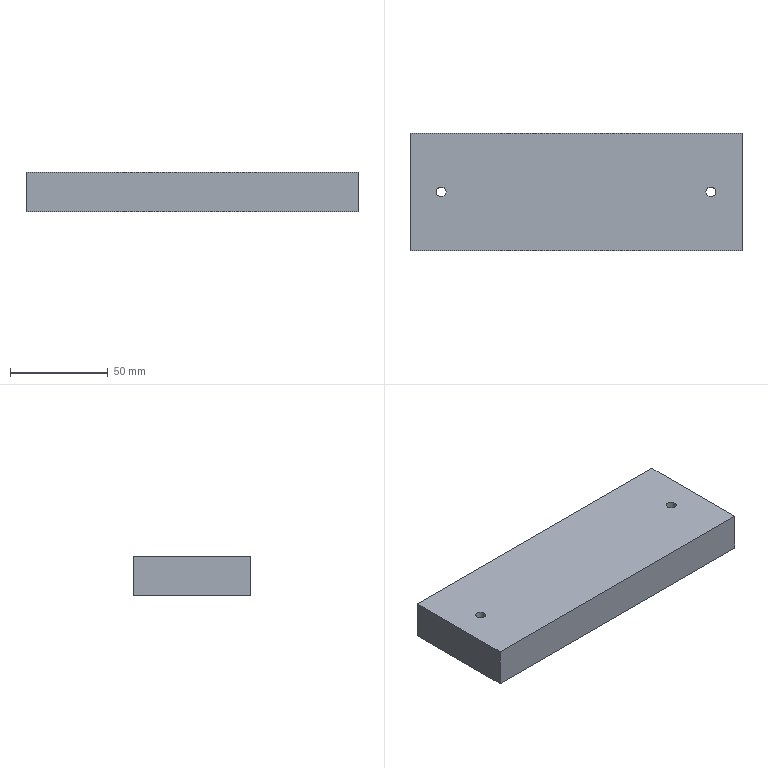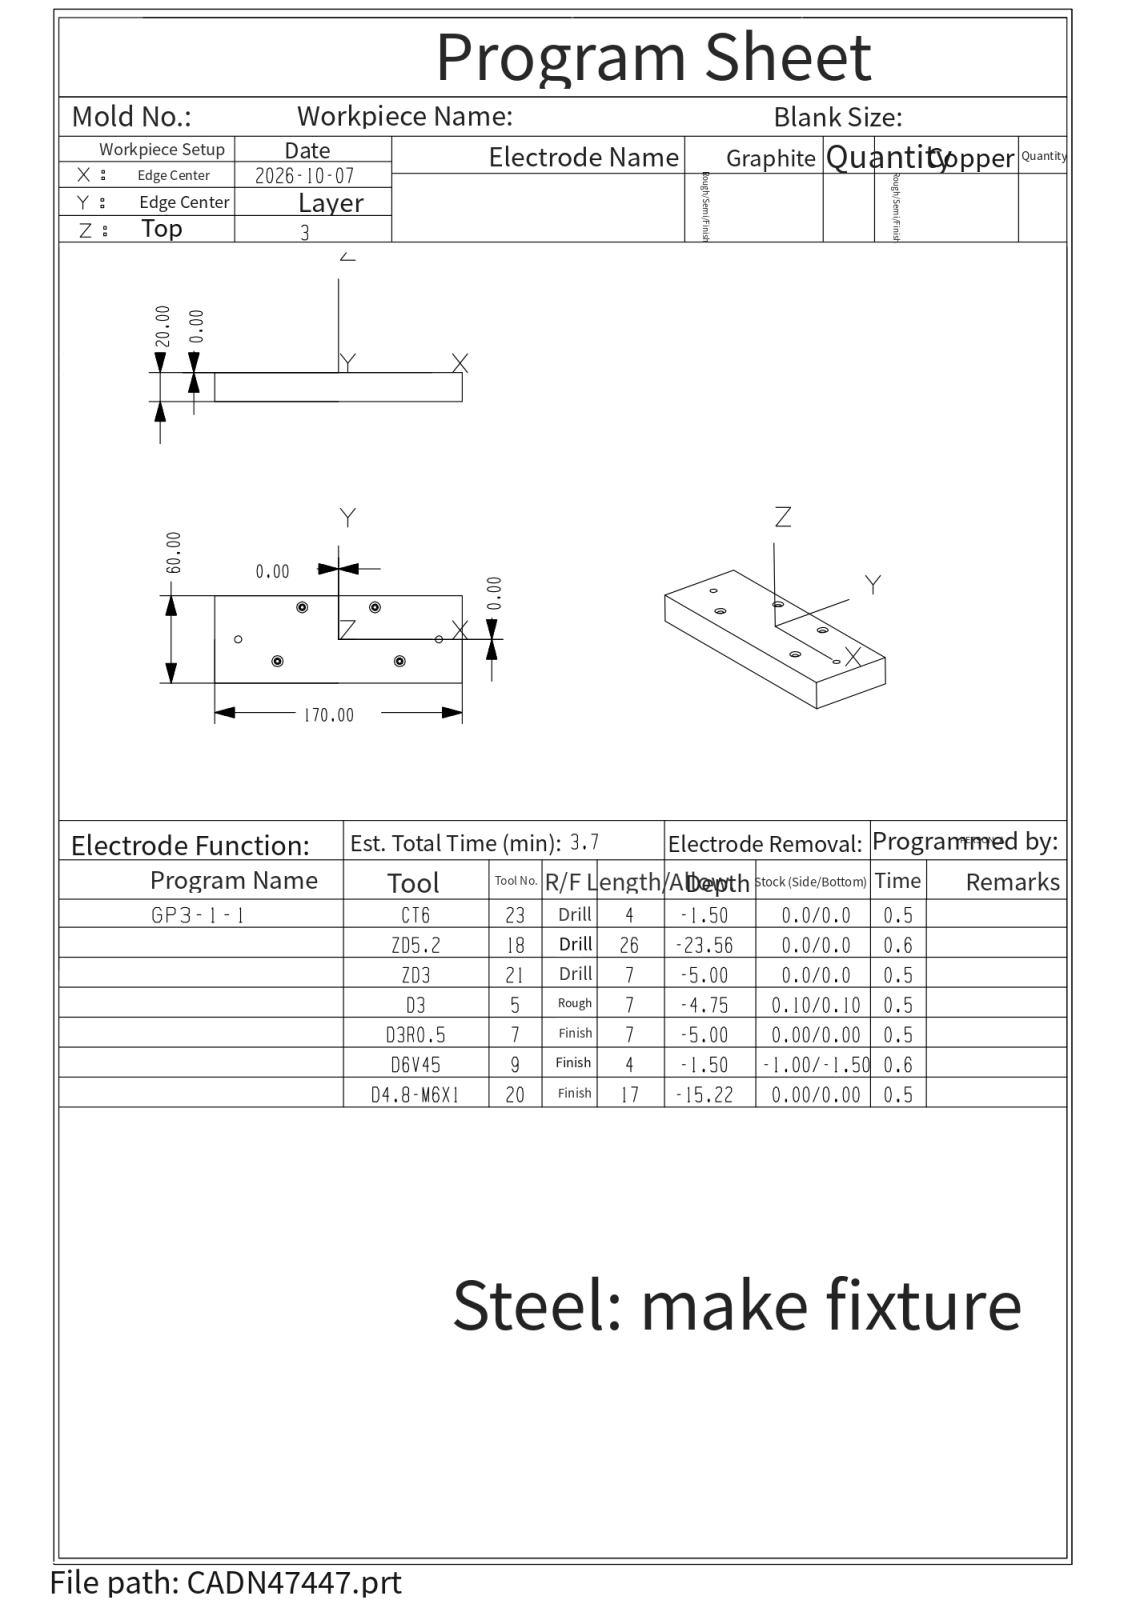NC program | NX | posted by the shop | part box 170 x 60 x 20 mm
Lines 60 to 1040 of 14163:
T05 M06
T07
( name=D3    T=5 )
( XY = 0.10 )
( Z = 0.10 )
G00 G90 G54 X43.611 Y-14.897 S5000 M03
G43 Z10. H05 M08
Z.2
G17 G01 X43.421 Y-14.198 Z.175 F1600.
X43.017 Y-13.724 Z.153
X42.217 Y-13.383 Z.123
X41.354 Y-13.502 Z.092
X40.676 Y-14.048 Z.062
X40.416 Y-14.613 Z.04
X40.389 Y-15.254 Z.018
X40.612 Y-15.855 Z-.005
X41.048 Y-16.325 Z-.027
X41.614 Y-16.585 Z-.049
X41.689 Y-16.601 Z-.052
X42.001 Z-.062
G03 I0.0 J1.601 F2000.
G01 X42.235 Y-16.576 Z-.067
X42.384 Y-16.541 Z-.069
X42.597 Y-16.463 Z-.073
X42.738 Y-16.391 Z-.076
X42.924 Y-16.266 Z-.08
X43.043 Y-16.162 Z-.083
X43.192 Y-15.997 Z-.087
X43.282 Y-15.869 Z-.09
X43.386 Y-15.675 Z-.094
X43.442 Y-15.53 Z-.097
X43.496 Y-15.318 Z-.101
X43.515 Y-15.165 Z-.103
X43.516 Y-14.948 Z-.107
X43.498 Y-14.796 Z-.11
X43.447 Y-14.588 Z-.114
X43.394 Y-14.445 Z-.117
X43.295 Y-14.256 Z-.121
X43.209 Y-14.132 Z-.124
X43.069 Y-13.974 Z-.128
X42.957 Y-13.875 Z-.131
X42.81 Y-13.772 Z-.134
X42.652 Y-13.687 Z-.137
G03 X42.001 Y-16.465 I-.651 J-1.313
G01 X42.256 Y-16.436 Z-.142
X42.406 Y-16.396 Z-.145
X42.629 Y-16.304 Z-.149
X42.772 Y-16.219 Z-.152
X42.958 Y-16.07 Z-.156
X43.073 Y-15.948 Z-.159
X43.208 Y-15.756 Z-.163
X43.284 Y-15.608 Z-.166
X43.361 Y-15.387 Z-.17
X43.392 Y-15.224 Z-.173
X43.404 Y-14.993 Z-.178
X43.389 Y-14.829 Z-.181
X43.336 Y-14.606 Z-.185
X43.277 Y-14.454 Z-.188
X43.165 Y-14.255 Z-.192
X43.067 Y-14.126 Z-.195
X42.905 Y-13.968 Z-.199
X42.776 Y-13.873 Z-.202
X42.577 Y-13.766 Z-.207
X42.428 Y-13.711 Z-.21
X42.21 Y-13.664 Z-.214
X42.052 Y-13.653 Z-.217
X41.863 Y-13.664 Z-.22
X41.677 Y-13.701 Z-.224
G03 X42.001 Y-16.339 I.324 J-1.299
G01 X42.251 Y-16.309 Z-.228
X42.392 Y-16.271 Z-.231
X42.607 Y-16.177 Z-.235
X42.743 Y-16.092 Z-.238
X42.918 Y-15.942 Z-.242
X43.025 Y-15.82 Z-.245
X43.147 Y-15.627 Z-.249
X43.212 Y-15.479 Z-.252
X43.272 Y-15.26 Z-.256
X43.291 Y-15.101 Z-.259
X43.284 Y-14.876 Z-.263
X43.255 Y-14.719 Z-.266
X43.183 Y-14.507 Z-.27
X43.11 Y-14.366 Z-.273
X42.979 Y-14.186 Z-.277
X42.869 Y-14.074 Z-.28
X42.692 Y-13.942 Z-.284
X42.554 Y-13.867 Z-.287
X42.348 Y-13.793 Z-.291
X42.195 Y-13.762 Z-.294
X41.978 Y-13.752 Z-.298
X41.824 Y-13.768 Z-.301
X41.614 Y-13.822 Z-.305
X41.473 Y-13.881 Z-.308
X41.289 Y-13.994 Z-.312
X41.172 Y-14.092 Z-.315
X41.05 Y-14.227 Z-.318
X40.948 Y-14.38 Z-.322
G03 X42.001 Y-16.222 I1.052 J-.62
G01 X42.255 Y-16.189 Z-.327
X42.395 Y-16.147 Z-.33
X42.608 Y-16.043 Z-.335
X42.74 Y-15.95 Z-.338
X42.906 Y-15.786 Z-.343
X43.001 Y-15.653 Z-.347
X43.104 Y-15.447 Z-.351
X43.151 Y-15.291 Z-.355
X43.181 Y-15.064 Z-.36
X43.175 Y-14.902 Z-.363
X43.129 Y-14.68 Z-.368
X43.072 Y-14.53 Z-.371
X42.958 Y-14.335 Z-.376
X42.855 Y-14.213 Z-.38
X42.685 Y-14.067 Z-.385
X42.549 Y-13.985 Z-.388
X42.343 Y-13.903 Z-.393
X42.188 Y-13.87 Z-.396
X41.968 Y-13.86 Z-.401
X41.813 Y-13.878 Z-.405
X41.602 Y-13.939 Z-.41
X41.462 Y-14.007 Z-.413
X41.284 Y-14.132 Z-.418
X41.174 Y-14.241 Z-.421
X41.064 Y-14.389 Z-.425
X40.979 Y-14.553 Z-.43
G03 X42.001 Y-16.115 I1.021 J-.447
G01 X42.253 Y-16.08 Z-.436
X42.389 Y-16.036 Z-.439
X42.597 Y-15.926 Z-.445
X42.723 Y-15.827 Z-.449
X42.875 Y-15.655 Z-.455
X42.96 Y-15.516 Z-.459
X43.041 Y-15.304 Z-.465
X43.072 Y-15.146 Z-.469
X43.074 Y-14.92 Z-.474
X43.047 Y-14.762 Z-.478
X42.97 Y-14.551 Z-.484
X42.89 Y-14.414 Z-.488
X42.745 Y-14.245 Z-.494
X42.622 Y-14.146 Z-.498
X42.429 Y-14.039 Z-.504
X42.281 Y-13.989 Z-.508
X42.064 Y-13.958 Z-.513
X41.908 Y-13.963 Z-.517
X41.696 Y-14.009 Z-.523
X41.553 Y-14.068 Z-.527
X41.372 Y-14.185 Z-.533
X41.26 Y-14.29 Z-.537
X41.148 Y-14.435 Z-.542
X41.064 Y-14.598 Z-.547
G03 X42.001 Y-16.019 I.936 J-.402
G01 X42.254 Y-15.981 Z-.554
X42.388 Y-15.933 Z-.558
X42.59 Y-15.815 Z-.565
X42.71 Y-15.708 Z-.57
X42.849 Y-15.525 Z-.576
X42.92 Y-15.38 Z-.581
X42.977 Y-15.16 Z-.588
X42.987 Y-14.999 Z-.592
X42.957 Y-14.776 Z-.599
X42.904 Y-14.624 Z-.604
X42.791 Y-14.431 Z-.61
X42.686 Y-14.312 Z-.615
X42.509 Y-14.178 Z-.622
X42.368 Y-14.109 Z-.627
X42.155 Y-14.053 Z-.633
X41.998 Y-14.044 Z-.638
X41.782 Y-14.074 Z-.645
X41.635 Y-14.124 Z-.649
X41.448 Y-14.234 Z-.656
X41.333 Y-14.336 Z-.661
X41.219 Y-14.481 Z-.667
X41.136 Y-14.645 Z-.672
G03 X42.001 Y-15.935 I.865 J-.355
G01 X42.258 Y-15.893 Z-.681
X42.391 Y-15.84 Z-.685
X42.59 Y-15.709 Z-.693
X42.703 Y-15.593 Z-.699
X42.826 Y-15.395 Z-.706
X42.88 Y-15.239 Z-.712
X42.908 Y-15.011 Z-.72
X42.892 Y-14.848 Z-.725
X42.821 Y-14.631 Z-.733
X42.739 Y-14.49 Z-.739
X42.584 Y-14.325 Z-.746
X42.452 Y-14.233 Z-.752
X42.244 Y-14.148 Z-.759
X42.086 Y-14.121 Z-.765
X41.863 Y-14.132 Z-.773
X41.71 Y-14.174 Z-.778
X41.514 Y-14.277 Z-.786
X41.393 Y-14.378 Z-.792
X41.277 Y-14.525 Z-.798
X41.194 Y-14.694 Z-.805
G03 X42.001 Y-15.863 I.807 J-.306
G01 X42.268 Y-15.816 Z-.815
X42.402 Y-15.756 Z-.82
X42.598 Y-15.606 Z-.829
X42.703 Y-15.476 Z-.836
X42.805 Y-15.257 Z-.845
X42.837 Y-15.09 Z-.851
X42.825 Y-14.852 Z-.86
X42.776 Y-14.69 Z-.866
X42.655 Y-14.487 Z-.875
X42.536 Y-14.368 Z-.882
X42.336 Y-14.247 Z-.891
X42.176 Y-14.197 Z-.897
X41.944 Y-14.184 Z-.906
X41.781 Y-14.215 Z-.913
X41.571 Y-14.311 Z-.922
X41.442 Y-14.414 Z-.928
X41.32 Y-14.567 Z-.936
X41.238 Y-14.746 Z-.943
G03 X42.001 Y-15.804 I.763 J-.254
G01 X42.254 Y-15.759 Z-.954
X42.379 Y-15.703 Z-.959
X42.564 Y-15.561 Z-.969
X42.662 Y-15.436 Z-.975
X42.756 Y-15.229 Z-.984
X42.785 Y-15.07 Z-.991
X42.769 Y-14.845 Z-1.
X42.719 Y-14.692 Z-1.007
X42.6 Y-14.503 Z-1.016
X42.484 Y-14.392 Z-1.023
X42.291 Y-14.283 Z-1.032
X42.138 Y-14.24 Z-1.039
X41.917 Y-14.236 Z-1.048
X41.763 Y-14.271 Z-1.055
X41.567 Y-14.371 Z-1.064
X41.449 Y-14.474 Z-1.071
X41.339 Y-14.625 Z-1.079
X41.27 Y-14.8 Z-1.087
G03 X42.001 Y-15.758 I.731 J-.2
G01 X42.244 Y-15.715 Z-1.097
X42.363 Y-15.661 Z-1.103
X42.54 Y-15.523 Z-1.113
X42.633 Y-15.403 Z-1.119
X42.721 Y-15.202 Z-1.129
X42.745 Y-15.049 Z-1.136
X42.726 Y-14.833 Z-1.145
X42.674 Y-14.687 Z-1.152
X42.553 Y-14.508 Z-1.161
X42.438 Y-14.405 Z-1.168
X42.247 Y-14.306 Z-1.178
X42.098 Y-14.271 Z-1.185
X41.884 Y-14.276 Z-1.194
X41.737 Y-14.317 Z-1.201
X41.552 Y-14.424 Z-1.21
X41.443 Y-14.53 Z-1.217
X41.346 Y-14.684 Z-1.225
X41.289 Y-14.857 Z-1.233
G03 X42.001 Y-15.726 I.712 J-.143
G01 X42.267 Y-15.674 Z-1.246
X42.392 Y-15.608 Z-1.252
X42.519 Y-15.503 Z-1.259
X42.572 Y-15.441 Z-1.263
X42.603 Y-15.396 Z-1.266
X42.656 Y-15.299 Z-1.271
X42.707 Y-15.138 Z-1.278
X42.717 Y-15.057 Z-1.282
X42.719 Y-15.004 Z-1.284
X42.711 Y-14.897 Z-1.289
X42.632 Y-14.661 Z-1.3
X42.541 Y-14.531 Z-1.308
X42.421 Y-14.423 Z-1.315
X42.355 Y-14.38 Z-1.319
X42.305 Y-14.355 Z-1.321
X42.2 Y-14.316 Z-1.326
X41.955 Y-14.29 Z-1.337
X41.799 Y-14.319 Z-1.345
X41.587 Y-14.425 Z-1.356
X41.465 Y-14.538 Z-1.363
X41.358 Y-14.708 Z-1.373
X41.303 Y-14.902 Z-1.382
G03 X42.001 Y-15.705 I.698 J-.098
G01 X42.26 Y-15.654 Z-1.394
X42.381 Y-15.591 Z-1.401
X42.555 Y-15.429 Z-1.412
X42.637 Y-15.29 Z-1.419
X42.696 Y-15.065 Z-1.43
X42.691 Y-14.9 Z-1.438
X42.618 Y-14.68 Z-1.448
X42.525 Y-14.544 Z-1.456
X42.346 Y-14.399 Z-1.467
X42.194 Y-14.336 Z-1.475
X41.967 Y-14.311 Z-1.486
X41.805 Y-14.339 Z-1.493
X41.601 Y-14.441 Z-1.504
X41.481 Y-14.552 Z-1.512
X41.377 Y-14.717 Z-1.521
X41.324 Y-14.905 Z-1.531
G03 X42.001 Y-15.684 I.677 J-.095
G01 X42.252 Y-15.634 Z-1.543
X42.369 Y-15.573 Z-1.549
X42.538 Y-15.416 Z-1.56
X42.618 Y-15.282 Z-1.568
X42.675 Y-15.064 Z-1.578
X42.67 Y-14.904 Z-1.586
X42.601 Y-14.691 Z-1.597
X42.51 Y-14.559 Z-1.605
X42.337 Y-14.418 Z-1.616
X42.19 Y-14.356 Z-1.623
X41.97 Y-14.331 Z-1.634
X41.813 Y-14.359 Z-1.642
X41.615 Y-14.456 Z-1.653
X41.498 Y-14.564 Z-1.66
X41.397 Y-14.723 Z-1.67
X41.345 Y-14.905 Z-1.679
G03 X42.001 Y-15.663 I.656 J-.095
G01 X42.244 Y-15.615 Z-1.691
X42.357 Y-15.556 Z-1.698
X42.521 Y-15.404 Z-1.709
X42.599 Y-15.274 Z-1.716
X42.654 Y-15.063 Z-1.727
X42.65 Y-14.908 Z-1.735
X42.583 Y-14.702 Z-1.746
X42.495 Y-14.574 Z-1.753
X42.328 Y-14.437 Z-1.764
X42.186 Y-14.377 Z-1.772
X41.973 Y-14.352 Z-1.783
X41.821 Y-14.378 Z-1.79
X41.629 Y-14.472 Z-1.801
X41.516 Y-14.575 Z-1.809
X41.417 Y-14.729 Z-1.818
X41.366 Y-14.905 Z-1.828
G03 X42.001 Y-15.642 I.635 J-.095
G01 X42.185 Y-15.614 Z-1.837
X42.267 Y-15.582 Z-1.841
X42.309 Y-15.561 Z-1.844
X42.388 Y-15.508 Z-1.849
X42.509 Y-15.385 Z-1.857
X42.555 Y-15.316 Z-1.862
X42.578 Y-15.269 Z-1.864
X42.614 Y-15.169 Z-1.87
X42.636 Y-15. Z-1.879
X42.63 Y-14.918 Z-1.883
X42.62 Y-14.866 Z-1.886
X42.588 Y-14.763 Z-1.891
X42.503 Y-14.617 Z-1.9
X42.449 Y-14.556 Z-1.904
X42.41 Y-14.52 Z-1.907
X42.323 Y-14.458 Z-1.912
X42.167 Y-14.393 Z-1.921
X42.088 Y-14.378 Z-1.925
X42.035 Y-14.373 Z-1.928
X41.929 Y-14.377 Z-1.934
X41.767 Y-14.419 Z-1.942
X41.694 Y-14.455 Z-1.946
X41.65 Y-14.483 Z-1.949
X41.568 Y-14.55 Z-1.955
X41.501 Y-14.628 Z-1.96
X41.448 Y-14.713 Z-1.966
X41.41 Y-14.805 Z-1.971
X41.387 Y-14.905 Z-1.976
G03 X42.001 Y-15.621 I.614 J-.095
G01 X42.178 Y-15.594 Z-1.985
X42.258 Y-15.563 Z-1.99
X42.299 Y-15.543 Z-1.992
X42.375 Y-15.492 Z-1.997
X42.492 Y-15.373 Z-2.006
X42.536 Y-15.306 Z-2.01
X42.559 Y-15.261 Z-2.013
X42.594 Y-15.164 Z-2.019
X42.615 Y-15.001 Z-2.027
X42.609 Y-14.922 Z-2.031
X42.6 Y-14.871 Z-2.034
X42.569 Y-14.772 Z-2.04
X42.488 Y-14.631 Z-2.048
X42.436 Y-14.571 Z-2.053
X42.398 Y-14.537 Z-2.055
X42.314 Y-14.477 Z-2.061
X42.164 Y-14.414 Z-2.07
X42.087 Y-14.399 Z-2.074
X42.036 Y-14.394 Z-2.077
X41.933 Y-14.397 Z-2.082
X41.777 Y-14.438 Z-2.091
X41.707 Y-14.472 Z-2.095
X41.664 Y-14.499 Z-2.098
X41.584 Y-14.563 Z-2.103
X41.519 Y-14.638 Z-2.109
X41.468 Y-14.72 Z-2.114
X41.431 Y-14.809 Z-2.119
X41.408 Y-14.905 Z-2.125
G03 X42.001 Y-15.6 I.593 J-.095
G01 X42.172 Y-15.574 Z-2.134
X42.249 Y-15.545 Z-2.138
X42.288 Y-15.524 Z-2.141
X42.362 Y-15.476 Z-2.146
X42.475 Y-15.361 Z-2.154
X42.518 Y-15.296 Z-2.159
X42.54 Y-15.252 Z-2.162
X42.574 Y-15.159 Z-2.167
X42.594 Y-15.002 Z-2.176
X42.589 Y-14.926 Z-2.18
X42.58 Y-14.877 Z-2.183
X42.55 Y-14.781 Z-2.188
X42.472 Y-14.644 Z-2.197
X42.422 Y-14.587 Z-2.201
X42.386 Y-14.554 Z-2.204
X42.305 Y-14.496 Z-2.21
X42.16 Y-14.435 Z-2.218
X42.086 Y-14.42 Z-2.222
X42.037 Y-14.415 Z-2.225
X41.938 Y-14.418 Z-2.231
X41.787 Y-14.456 Z-2.239
X41.719 Y-14.489 Z-2.244
X41.677 Y-14.515 Z-2.246
X41.601 Y-14.577 Z-2.252
X41.538 Y-14.648 Z-2.257
X41.488 Y-14.727 Z-2.263
X41.452 Y-14.812 Z-2.268
X41.429 Y-14.905 Z-2.273
G03 X42.001 Y-15.58 I.572 J-.095
G01 X42.166 Y-15.554 Z-2.282
X42.278 Y-15.506 Z-2.289
X42.349 Y-15.459 Z-2.294
X42.458 Y-15.349 Z-2.303
X42.499 Y-15.287 Z-2.307
X42.521 Y-15.244 Z-2.31
X42.553 Y-15.155 Z-2.316
X42.573 Y-15.003 Z-2.324
X42.568 Y-14.93 Z-2.328
X42.56 Y-14.882 Z-2.331
X42.532 Y-14.79 Z-2.337
X42.456 Y-14.658 Z-2.345
X42.408 Y-14.603 Z-2.35
X42.373 Y-14.571 Z-2.352
X42.295 Y-14.515 Z-2.358
X42.156 Y-14.455 Z-2.367
X42.085 Y-14.441 Z-2.371
X42.038 Y-14.436 Z-2.374
X41.943 Y-14.438 Z-2.379
X41.797 Y-14.475 Z-2.388
X41.731 Y-14.506 Z-2.392
X41.691 Y-14.53 Z-2.395
X41.617 Y-14.59 Z-2.401
X41.508 Y-14.734 Z-2.411
X41.45 Y-14.906 Z-2.422
G03 X42.001 Y-15.559 I.551 J-.094
G01 X42.186 Y-15.525 Z-2.432
X42.266 Y-15.489 Z-2.438
X42.307 Y-15.464 Z-2.441
X42.382 Y-15.404 Z-2.447
X42.487 Y-15.265 Z-2.456
X42.52 Y-15.189 Z-2.461
X42.536 Y-15.139 Z-2.465
X42.552 Y-15.032 Z-2.471
X42.533 Y-14.862 Z-2.481
X42.507 Y-14.785 Z-2.486
X42.483 Y-14.737 Z-2.489
X42.421 Y-14.648 Z-2.496
X42.292 Y-14.537 Z-2.506
X42.22 Y-14.5 Z-2.511
X42.17 Y-14.481 Z-2.514
X42.065 Y-14.459 Z-2.521
X41.895 Y-14.467 Z-2.531
X41.818 Y-14.489 Z-2.536
X41.77 Y-14.51 Z-2.539
X41.678 Y-14.565 Z-2.546
X41.602 Y-14.635 Z-2.552
X41.542 Y-14.716 Z-2.558
X41.498 Y-14.806 Z-2.564
X41.471 Y-14.906 Z-2.57
G03 X42.001 Y-15.538 I.529 J-.094
G01 X42.179 Y-15.506 Z-2.581
X42.256 Y-15.471 Z-2.586
X42.295 Y-15.447 Z-2.589
X42.367 Y-15.389 Z-2.595
X42.468 Y-15.256 Z-2.605
X42.5 Y-15.183 Z-2.61
X42.515 Y-15.134 Z-2.613
X42.531 Y-15.032 Z-2.62
X42.514 Y-14.868 Z-2.63
X42.488 Y-14.794 Z-2.635
X42.465 Y-14.748 Z-2.638
X42.406 Y-14.663 Z-2.645
X42.282 Y-14.556 Z-2.654
X42.214 Y-14.52 Z-2.659
X42.166 Y-14.502 Z-2.663
X42.065 Y-14.48 Z-2.669
X41.902 Y-14.487 Z-2.679
X41.828 Y-14.508 Z-2.684
X41.781 Y-14.527 Z-2.687
X41.693 Y-14.58 Z-2.694
X41.62 Y-14.647 Z-2.7
X41.562 Y-14.724 Z-2.706
X41.519 Y-14.81 Z-2.713
X41.493 Y-14.906 Z-2.719
G03 X42.001 Y-15.517 I.508 J-.094
G01 X42.172 Y-15.486 Z-2.729
X42.245 Y-15.453 Z-2.735
X42.283 Y-15.43 Z-2.738
X42.352 Y-15.374 Z-2.744
X42.45 Y-15.246 Z-2.754
X42.481 Y-15.177 Z-2.759
X42.495 Y-15.13 Z-2.762
X42.51 Y-15.032 Z-2.768
X42.494 Y-14.875 Z-2.778
X42.469 Y-14.804 Z-2.783
X42.448 Y-14.76 Z-2.786
X42.391 Y-14.678 Z-2.793
X42.273 Y-14.574 Z-2.803
X42.207 Y-14.54 Z-2.808
X42.161 Y-14.522 Z-2.811
X42.064 Y-14.501 Z-2.818
X41.909 Y-14.507 Z-2.828
X41.838 Y-14.526 Z-2.833
X41.792 Y-14.545 Z-2.836
X41.708 Y-14.595 Z-2.843
X41.637 Y-14.659 Z-2.849
X41.581 Y-14.732 Z-2.855
X41.54 Y-14.814 Z-2.861
X41.514 Y-14.906 Z-2.867
G03 X42.001 Y-15.496 I.487 J-.094
G01 X42.164 Y-15.467 Z-2.878
X42.235 Y-15.435 Z-2.883
X42.271 Y-15.413 Z-2.886
X42.337 Y-15.36 Z-2.892
X42.431 Y-15.237 Z-2.902
X42.461 Y-15.171 Z-2.907
X42.474 Y-15.126 Z-2.91
X42.489 Y-15.032 Z-2.917
X42.474 Y-14.882 Z-2.927
X42.451 Y-14.814 Z-2.932
X42.43 Y-14.771 Z-2.935
X42.376 Y-14.692 Z-2.942
X42.264 Y-14.593 Z-2.952
X42.201 Y-14.56 Z-2.956
X42.157 Y-14.543 Z-2.96
X42.064 Y-14.522 Z-2.966
X41.915 Y-14.527 Z-2.976
X41.847 Y-14.545 Z-2.981
X41.804 Y-14.563 Z-2.985
X41.723 Y-14.61 Z-2.991
X41.655 Y-14.671 Z-2.997
X41.601 Y-14.74 Z-3.004
X41.561 Y-14.819 Z-3.01
X41.535 Y-14.906 Z-3.016
G03 X42.001 Y-15.475 I.466 J-.094
G01 X42.157 Y-15.447 Z-3.027
X42.225 Y-15.417 Z-3.032
X42.259 Y-15.396 Z-3.035
X42.323 Y-15.345 Z-3.041
X42.412 Y-15.228 Z-3.051
X42.441 Y-15.165 Z-3.056
X42.454 Y-15.122 Z-3.059
X42.468 Y-15.032 Z-3.065
X42.454 Y-14.888 Z-3.075
X42.432 Y-14.823 Z-3.08
X42.413 Y-14.783 Z-3.084
X42.362 Y-14.707 Z-3.09
X42.254 Y-14.612 Z-3.1
X42.194 Y-14.58 Z-3.105
X42.153 Y-14.563 Z-3.108
X42.064 Y-14.543 Z-3.115
X41.922 Y-14.547 Z-3.125
X41.857 Y-14.564 Z-3.13
X41.815 Y-14.58 Z-3.133
X41.738 Y-14.626 Z-3.14
X41.672 Y-14.683 Z-3.146
X41.62 Y-14.749 Z-3.152
X41.581 Y-14.823 Z-3.158
X41.556 Y-14.907 Z-3.164
G03 X42.001 Y-15.454 I.445 J-.093
G01 X42.179 Y-15.416 Z-3.177
X42.252 Y-15.375 Z-3.183
X42.289 Y-15.347 Z-3.187
X42.353 Y-15.28 Z-3.194
X42.43 Y-15.13 Z-3.206
X42.445 Y-15.054 Z-3.212
X42.448 Y-15.003 Z-3.216
X42.435 Y-14.899 Z-3.224
X42.367 Y-14.749 Z-3.236
X42.318 Y-14.69 Z-3.242
X42.28 Y-14.656 Z-3.246
X42.191 Y-14.601 Z-3.254
X42.032 Y-14.561 Z-3.265
X41.956 Y-14.563 Z-3.271
X41.906 Y-14.572 Z-3.275
X41.808 Y-14.607 Z-3.283
X41.725 Y-14.662 Z-3.291
X41.659 Y-14.73 Z-3.298
X41.609 Y-14.812 Z-3.306
X41.578 Y-14.907 Z-3.313
G03 X42.001 Y-15.433 I.423 J-.093
G01 X42.171 Y-15.397 Z-3.326
X42.24 Y-15.358 Z-3.332
X42.275 Y-15.332 Z-3.336
X42.336 Y-15.268 Z-3.343
X42.41 Y-15.125 Z-3.355
X42.424 Y-15.053 Z-3.36
X42.427 Y-15.004 Z-3.364
X42.415 Y-14.906 Z-3.372
X42.351 Y-14.762 Z-3.384
X42.305 Y-14.706 Z-3.39
X42.268 Y-14.674 Z-3.394
X42.184 Y-14.621 Z-3.402
X42.033 Y-14.582 Z-3.414
X41.962 Y-14.583 Z-3.42
X41.914 Y-14.591 Z-3.424
X41.821 Y-14.624 Z-3.432
X41.741 Y-14.676 Z-3.439
X41.678 Y-14.74 Z-3.447
X41.63 Y-14.817 Z-3.454
X41.599 Y-14.907 Z-3.462
G03 X42.001 Y-15.413 I.402 J-.093
G01 X42.162 Y-15.378 Z-3.474
X42.228 Y-15.341 Z-3.48
X42.261 Y-15.316 Z-3.484
X42.319 Y-15.256 Z-3.491
X42.389 Y-15.12 Z-3.503
X42.403 Y-15.052 Z-3.509
X42.406 Y-15.005 Z-3.513
X42.395 Y-14.912 Z-3.521
X42.335 Y-14.776 Z-3.533
X42.291 Y-14.723 Z-3.539
X42.257 Y-14.691 Z-3.543
X42.177 Y-14.641 Z-3.551
X42.035 Y-14.603 Z-3.562
X41.967 Y-14.604 Z-3.568
X41.921 Y-14.611 Z-3.572
X41.833 Y-14.641 Z-3.58
X41.757 Y-14.689 Z-3.588
X41.697 Y-14.75 Z-3.595
X41.651 Y-14.822 Z-3.603
X41.62 Y-14.907 Z-3.61
G03 X42.001 Y-15.392 I.381 J-.093
G01 X42.153 Y-15.359 Z-3.623
X42.215 Y-15.324 Z-3.629
X42.247 Y-15.301 Z-3.633
X42.302 Y-15.243 Z-3.64
X42.369 Y-15.116 Z-3.652
X42.382 Y-15.051 Z-3.658
X42.385 Y-15.007 Z-3.662
X42.375 Y-14.919 Z-3.669
X42.319 Y-14.789 Z-3.681
X42.278 Y-14.739 Z-3.687
X42.246 Y-14.709 Z-3.691
X42.171 Y-14.661 Z-3.699
X42.036 Y-14.624 Z-3.711
X41.972 Z-3.717
X41.929 Y-14.631 Z-3.721
X41.845 Y-14.659 Z-3.729
X41.773 Y-14.703 Z-3.736
X41.716 Y-14.76 Z-3.744
X41.671 Y-14.828 Z-3.751
X41.642 Y-14.908 Z-3.759
G03 X42.001 Y-15.371 I.359 J-.092
G01 X42.18 Y-15.322 Z-3.774
X42.245 Y-15.275 Z-3.782
X42.277 Y-15.241 Z-3.786
X42.329 Y-15.162 Z-3.796
X42.364 Y-14.996 Z-3.81
X42.355 Y-14.922 Z-3.818
X42.339 Y-14.872 Z-3.823
X42.287 Y-14.781 Z-3.833
X42.157 Y-14.678 Z-3.847
X42.088 Y-14.654 Z-3.854
X42.038 Y-14.645 Z-3.86
X41.932 Y-14.652 Z-3.87
X41.838 Y-14.686 Z-3.879
X41.762 Y-14.741 Z-3.889
X41.703 Y-14.814 Z-3.898
X41.663 Y-14.908 Z-3.907
G03 X42.001 Y-15.35 I.338 J-.092
G01 X42.169 Y-15.304 Z-3.923
X42.23 Y-15.26 Z-3.93
X42.261 Y-15.229 Z-3.935
X42.309 Y-15.154 Z-3.944
X42.343 Y-14.998 Z-3.959
X42.335 Y-14.928 Z-3.966
X42.321 Y-14.882 Z-3.971
X42.272 Y-14.796 Z-3.981
X42.151 Y-14.698 Z-3.996
X42.087 Y-14.675 Z-4.003
X42.039 Y-14.666 Z-4.008
X41.94 Y-14.671 Z-4.019
X41.851 Y-14.703 Z-4.028
X41.779 Y-14.753 Z-4.037
X41.723 Y-14.821 Z-4.046
X41.685 Y-14.909 Z-4.056
G03 X42.001 Y-15.329 I.316 J-.091
G01 X42.158 Y-15.286 Z-4.071
X42.215 Y-15.245 Z-4.079
X42.244 Y-15.216 Z-4.084
X42.29 Y-15.146 Z-4.093
X42.323 Y-15. Z-4.107
X42.315 Y-14.935 Z-4.115
X42.302 Y-14.892 Z-4.12
X42.257 Y-14.811 Z-4.13
X42.145 Y-14.718 Z-4.144
X42.085 Y-14.696 Z-4.152
X42.04 Y-14.688 Z-4.157
X41.948 Y-14.691 Z-4.167
X41.865 Y-14.719 Z-4.176
X41.797 Y-14.765 Z-4.186
X41.743 Y-14.828 Z-4.195
X41.706 Y-14.909 Z-4.204
G03 X42.001 Y-15.308 I.294 J-.091
G01 X42.147 Y-15.269 Z-4.22
X42.201 Y-15.23 Z-4.227
X42.228 Y-15.203 Z-4.232
X42.271 Y-15.138 Z-4.241
X42.302 Y-15.002 Z-4.256
X42.295 Y-14.942 Z-4.263
X42.283 Y-14.901 Z-4.268
X42.242 Y-14.826 Z-4.278
X42.139 Y-14.738 Z-4.293
X42.083 Y-14.717 Z-4.3
X42.042 Y-14.709 Z-4.305
X41.956 Y-14.711 Z-4.316
X41.878 Y-14.736 Z-4.325
X41.815 Y-14.778 Z-4.334
X41.764 Y-14.835 Z-4.343
X41.728 Y-14.91 Z-4.353
G03 X42.001 Y-15.287 I.273 J-.09
G01 X42.18 Y-15.221 Z-4.372
X42.229 Y-15.167 Z-4.382
X42.253 Y-15.126 Z-4.389
X42.276 Y-15.055 Z-4.399
X42.279 Y-15.032 Z-4.402
X42.236 Y-14.853 Z-4.422
X42.19 Y-14.799 Z-4.431
X42.153 Y-14.77 Z-4.438
X42.085 Y-14.74 Z-4.448
X42.063 Y-14.734 Z-4.452
X41.959 Y-14.732 Z-4.464
X41.873 Y-14.762 Z-4.477
X41.803 Y-14.82 Z-4.489
X41.75 Y-14.911 Z-4.501
G03 X42.001 Y-15.266 I.251 J-.089
G01 X42.164 Y-15.207 Z-4.518
X42.21 Y-15.159 Z-4.526
X42.233 Y-15.122 Z-4.532
X42.259 Y-15.037 Z-4.543
X42.231 Y-14.882 Z-4.558
X42.195 Y-14.831 Z-4.566
X42.16 Y-14.799 Z-4.572
X42.096 Y-14.764 Z-4.581
X42.072 Y-14.757 Z-4.584
X41.979 Y-14.75 Z-4.595
X41.901 Y-14.773 Z-4.605
X41.833 Y-14.821 Z-4.616
X41.78 Y-14.9 Z-4.626
G03 X42.001 Y-15.242 I.221 J-.1
G01 X41.794 Y-15.06 Z-4.688
X41.958 Y-14.831 Z-4.751
G03 I.043 J-.169
G01 Z-3.751
G00 Z10.
X23.395 Y21.889
Z.2
G01 X23.389 Y21.746 Z.195 F1600.
X23.612 Y21.145 Z.173
X24.048 Y20.675 Z.15
X24.614 Y20.415 Z.128
X25.337 Y20.404 Z.103
X25.911 Y20.646 Z.081
X26.447 Y21.245 Z.053
X26.632 Y22.027 Z.025
X26.421 Y22.802 Z-.003
X26.017 Y23.276 Z-.024
X25.312 Y23.601 Z-.052
X25.001 Z-.062
G03 I0.0 J-1.601 F2000.
G01 X24.766 Y23.576 Z-.067
X24.618 Y23.541 Z-.069
X24.404 Y23.463 Z-.073
X24.263 Y23.391 Z-.076
X24.078 Y23.266 Z-.08
X23.958 Y23.162 Z-.083
X23.81 Y22.997 Z-.087
X23.719 Y22.869 Z-.09
X23.616 Y22.675 Z-.094
X23.559 Y22.53 Z-.097
X23.506 Y22.318 Z-.101
X23.486 Y22.165 Z-.103
X23.485 Y21.948 Z-.107
X23.503 Y21.796 Z-.11
X23.554 Y21.588 Z-.114
X23.608 Y21.445 Z-.117
X23.707 Y21.256 Z-.121
X23.792 Y21.132 Z-.124
X23.933 Y20.974 Z-.128
X24.045 Y20.875 Z-.131
X24.191 Y20.772 Z-.134
X24.35 Y20.687 Z-.137
G03 X25.001 Y23.465 I.651 J1.313
G01 X24.746 Y23.436 Z-.142
X24.596 Y23.396 Z-.145
X24.373 Y23.304 Z-.149
X24.229 Y23.219 Z-.152
X24.044 Y23.07 Z-.156
X23.929 Y22.948 Z-.159
X23.793 Y22.756 Z-.163
X23.717 Y22.608 Z-.166
X23.641 Y22.387 Z-.17
X23.609 Y22.224 Z-.173
X23.598 Y21.993 Z-.178
X23.613 Y21.829 Z-.181
X23.665 Y21.606 Z-.185
X23.725 Y21.454 Z-.188
X23.837 Y21.255 Z-.192
X23.935 Y21.126 Z-.195
X24.097 Y20.968 Z-.199
X24.226 Y20.873 Z-.202
X24.424 Y20.766 Z-.207
X24.574 Y20.711 Z-.21
X24.792 Y20.664 Z-.214
X24.95 Y20.653 Z-.217
X25.139 Y20.664 Z-.22
X25.325 Y20.701 Z-.224
G03 X25.001 Y23.339 I-.324 J1.299
G01 X24.75 Y23.309 Z-.228
X24.61 Y23.271 Z-.231
X24.395 Y23.177 Z-.235
X24.258 Y23.092 Z-.238
X24.083 Y22.942 Z-.242
X23.977 Y22.82 Z-.245
X23.855 Y22.627 Z-.249
X23.789 Y22.479 Z-.252
X23.729 Y22.26 Z-.256
X23.711 Y22.101 Z-.259
X23.718 Y21.876 Z-.263
X23.746 Y21.719 Z-.266
X23.819 Y21.507 Z-.27
X23.892 Y21.366 Z-.273
X24.022 Y21.186 Z-.277
X24.133 Y21.074 Z-.28
X24.31 Y20.942 Z-.284
X24.447 Y20.867 Z-.287
X24.654 Y20.793 Z-.291
X24.806 Y20.762 Z-.294
X25.024 Y20.752 Z-.298
X25.178 Y20.768 Z-.301
X25.388 Y20.822 Z-.305
X25.529 Y20.881 Z-.308
X25.713 Y20.994 Z-.312
X25.829 Y21.092 Z-.315
X25.952 Y21.227 Z-.318
X26.053 Y21.38 Z-.322
G03 X25.001 Y23.222 I-1.052 J.62
G01 X24.747 Y23.189 Z-.327
X24.607 Y23.147 Z-.33
X24.394 Y23.043 Z-.335
X24.261 Y22.95 Z-.338
X24.096 Y22.786 Z-.343
X24. Y22.653 Z-.347
X23.898 Y22.447 Z-.351
X23.851 Y22.291 Z-.355
X23.821 Y22.064 Z-.36
X23.827 Y21.902 Z-.363
X23.872 Y21.68 Z-.368
X23.93 Y21.53 Z-.371
X24.044 Y21.335 Z-.376
X24.147 Y21.213 Z-.38
X24.317 Y21.067 Z-.385
X24.453 Y20.985 Z-.388
X24.659 Y20.903 Z-.393
X24.813 Y20.87 Z-.396
X25.034 Y20.86 Z-.401
X25.189 Y20.878 Z-.405
X25.399 Y20.939 Z-.41
X25.54 Y21.007 Z-.413
X25.717 Y21.132 Z-.418
X25.827 Y21.241 Z-.421
X25.938 Y21.389 Z-.425
X26.022 Y21.553 Z-.43
G03 X25.001 Y23.115 I-1.021 J.447
G01 X24.749 Y23.08 Z-.436
X24.612 Y23.036 Z-.439
X24.405 Y22.926 Z-.445
X24.279 Y22.827 Z-.449
X24.126 Y22.655 Z-.455
X24.042 Y22.516 Z-.459
X23.96 Y22.304 Z-.465
X23.93 Y22.146 Z-.469
X23.928 Y21.92 Z-.474
X23.955 Y21.762 Z-.478
X24.032 Y21.551 Z-.484
X24.112 Y21.414 Z-.488
X24.257 Y21.245 Z-.494
X24.379 Y21.146 Z-.498
X24.572 Y21.039 Z-.504
X24.721 Y20.989 Z-.508
X24.938 Y20.958 Z-.513
X25.093 Y20.963 Z-.517
X25.306 Y21.009 Z-.523
X25.448 Y21.068 Z-.527
X25.63 Y21.185 Z-.533
X25.742 Y21.29 Z-.537
X25.853 Y21.435 Z-.542
X25.937 Y21.598 Z-.547
G03 X25.001 Y23.019 I-.936 J.402
G01 X24.748 Y22.981 Z-.554
X24.614 Y22.933 Z-.558
X24.411 Y22.815 Z-.565
X24.292 Y22.708 Z-.57
X24.153 Y22.525 Z-.576
X24.082 Y22.38 Z-.581
X24.024 Y22.16 Z-.588
X24.015 Y21.999 Z-.592
X24.045 Y21.776 Z-.599
X24.097 Y21.624 Z-.604
X24.21 Y21.431 Z-.61
X24.316 Y21.312 Z-.615
X24.492 Y21.178 Z-.622
X24.634 Y21.109 Z-.627
X24.847 Y21.053 Z-.633
X25.003 Y21.044 Z-.638
X25.22 Y21.074 Z-.645
X25.366 Y21.124 Z-.649
X25.553 Y21.234 Z-.656
X25.669 Y21.336 Z-.661
X25.782 Y21.481 Z-.667
X25.866 Y21.645 Z-.672
G03 X25.001 Y22.935 I-.865 J.355
G01 X24.743 Y22.893 Z-.681
X24.61 Y22.84 Z-.685
X24.411 Y22.709 Z-.693
X24.298 Y22.593 Z-.699
X24.176 Y22.395 Z-.706
X24.121 Y22.239 Z-.712
X24.094 Y22.011 Z-.72
X24.11 Y21.848 Z-.725
X24.18 Y21.631 Z-.733
X24.263 Y21.49 Z-.739
X24.417 Y21.325 Z-.746
X24.55 Y21.233 Z-.752
X24.758 Y21.148 Z-.759
X24.916 Y21.121 Z-.765
X25.139 Y21.132 Z-.773
X25.292 Y21.174 Z-.778
X25.488 Y21.277 Z-.786
X25.608 Y21.378 Z-.792
X25.725 Y21.525 Z-.798
X25.808 Y21.694 Z-.805
G03 X25.001 Y22.863 I-.807 J.306
G01 X24.734 Y22.816 Z-.815
X24.6 Y22.756 Z-.82
X24.403 Y22.606 Z-.829
X24.298 Y22.476 Z-.836
X24.197 Y22.257 Z-.845
X24.164 Y22.09 Z-.851
X24.176 Y21.852 Z-.86
X24.226 Y21.69 Z-.866
X24.347 Y21.487 Z-.875
X24.466 Y21.368 Z-.882
X24.666 Y21.247 Z-.891
X24.826 Y21.197 Z-.897
X25.058 Y21.184 Z-.906
X25.221 Y21.215 Z-.913
X25.431 Y21.311 Z-.922
X25.559 Y21.414 Z-.928
X25.681 Y21.567 Z-.936
X25.763 Y21.746 Z-.943
G03 X25.001 Y22.804 I-.763 J.254
G01 X24.748 Y22.759 Z-.954
X24.622 Y22.703 Z-.959
X24.438 Y22.561 Z-.969
X24.339 Y22.436 Z-.975
X24.245 Y22.229 Z-.984
X24.217 Y22.07 Z-.991
X24.232 Y21.845 Z-1.
X24.282 Y21.692 Z-1.007
X24.402 Y21.503 Z-1.016
X24.517 Y21.392 Z-1.023
X24.711 Y21.283 Z-1.032
X24.864 Y21.24 Z-1.039
X25.085 Y21.236 Z-1.048
X25.239 Y21.271 Z-1.055
X25.435 Y21.371 Z-1.064
X25.553 Y21.474 Z-1.071
X25.663 Y21.625 Z-1.079
X25.732 Y21.8 Z-1.087
G03 X25.001 Y22.758 I-.731 J.2
G01 X24.757 Y22.715 Z-1.097
X24.638 Y22.661 Z-1.103
X24.462 Y22.523 Z-1.113
X24.369 Y22.403 Z-1.119
X24.281 Y22.202 Z-1.129
X24.256 Y22.049 Z-1.136